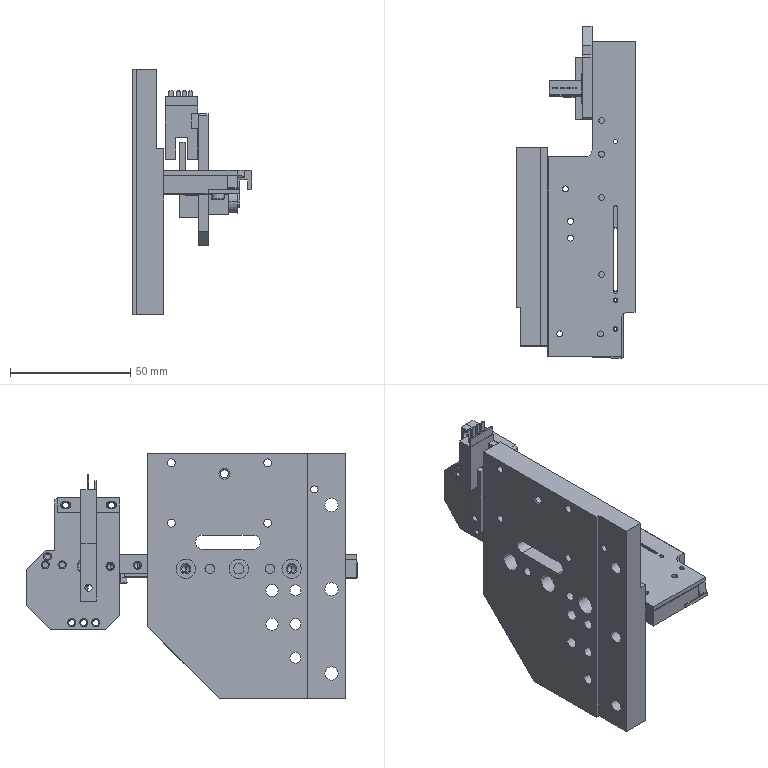Part | NX | 17 solids | 1220 faces | box 49.55 x 138 x 102 mm | volume 129003 mm3 | plane 864 | cylinder 224 | cone 124 | torus 8 | commonest cylinder face diameters 2.5 x55 3 x22 5.5 x18 1.5 x15 3.3 x14 4 x14